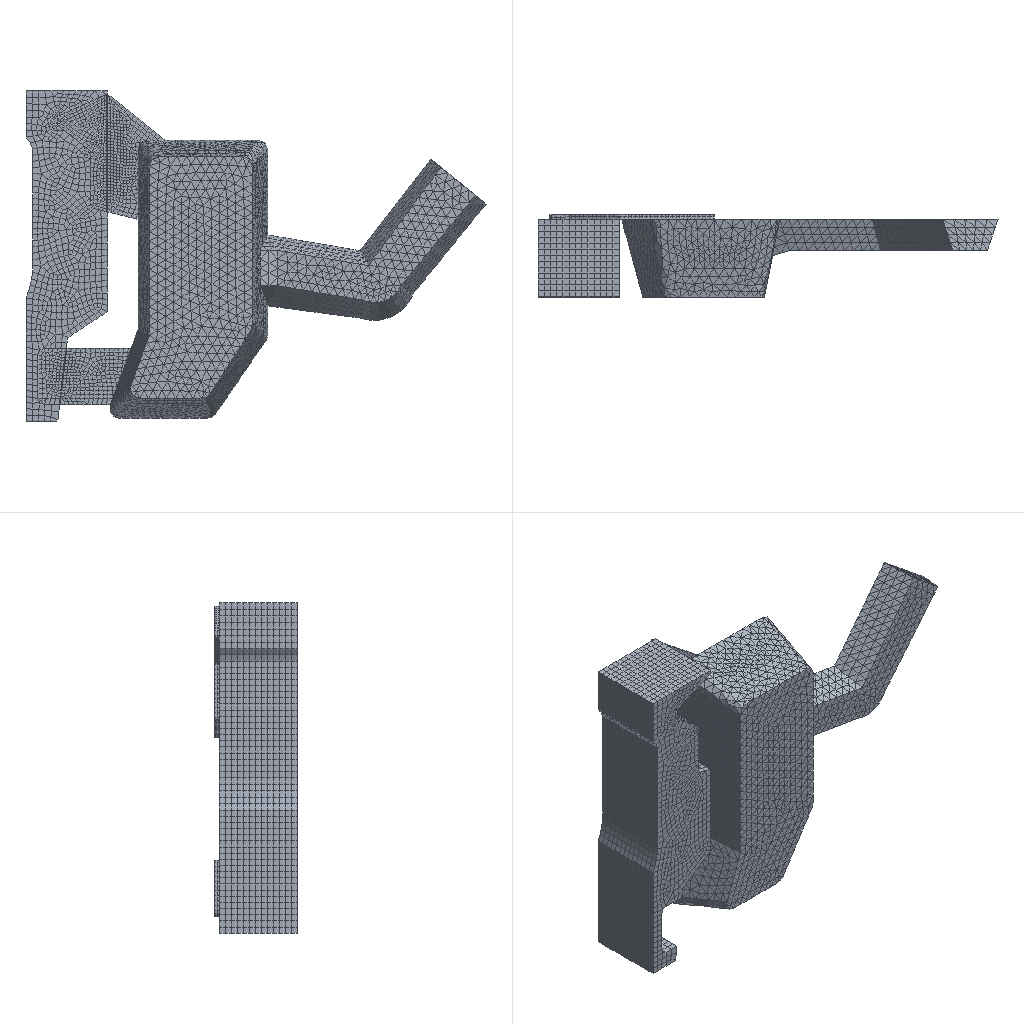Simulation study | abaqus
Set-up summary:
category,name,step,type,value,unit,region
solver,abaqus
solver,version,,,Abaqus/Explicit 2020
units,not stated in the deck,,not stated
analysis,deck,,transient,transient
load_step,Step-1,Step-1,transient,nlgeom=True
contact,interactions,,,general=1 pairs=0 ties=1
load_step,requested,,,1
mesh,nodes,,,20127
mesh,elements,,,40173
element_type,C3D4,,solid,29634
element_type,C3D8R,,solid,10483
element_type,COH3D8,,cohesive,56
load,load commands in deck,,count,1
bc,support commands in deck,,count,1
material,COH,,in results
material,MATERIAL-1,,in results
check,setup vs results,,match,"per instance, exact: element labels, types and connectivity; labels of the nodes the elements use; coordinates of those nodes at SINGLE_PRECISION in 2 of 3 instance(s)"
Abaqus input file, long lists of numbers shortened:
*Heading
** Job name: Job-1 Model name: Model-1
** Generated by: Abaqus/CAE 2020
*Preprint, echo=NO, model=NO, history=NO, contact=NO
**
** PARTS
**
*Part, name=work-1
*Node
      1,   552.966,         -10.,  -325.771
      2,   525.562,         -10.,  -321.176
** (6112 more lines like these left out)
*Element, type=C3D4
    1, 2263, 2264, 2265, 2266
    2, 2267, 2268, 2269, 2270
** (29632 more lines like these left out)
*Nset, nset=Set-4, generate
    1,  6114,     1
*Elset, elset=Set-4, generate
     1,  29634,      1
** Section: Section-1
*Solid Section, elset=Set-4, material=Material-1
,
*End Part
**
*Part, name=work-1-Copy
*Node
      1,   470.855,  0.8617,    -259.659
      2,   470.854,  0.8617,  -297.385
** (4547 more lines like these left out)
*Element, type=C3D8R
 1, 4472, 4473,  197,    7, 4475, 4474,  159,    4
 2, 4473, 4476,  198,  197, 4474, 4477,  158,  159
** (2694 more lines like these left out)
*Element, type=COH3D8
2697,   14,  358,  324,   13, 4437, 4436, 4435, 4434
2698,  358,  359,  323,  324, 4436, 4439, 4438, 4435
** (54 more lines like these left out)
*Nset, nset=Set-8, generate
    1,  4549,     1
*Elset, elset=Set-8, generate
    1,  2696,     1
*Elset, elset=CohesiveSeam-1-Elements, generate
 2697,  2752,     1
*Nset, nset=CohesiveSeam-1-TopNodes, generate
 4434,  4549,     1
*Nset, nset=CohesiveSeam-1-BottomNodes
   1,   2,   5,   8,  13,  14,  17,  18,  21,  86,  87,  88,  89,  90,  91,  92
  93,  94,  95,  96,  97,  98,  99, 100, 101, 102, 103, 104, 105, 106, 107, 108
** (6 more lines like these left out)
*Elset, elset=__PickedSurf18_S1, internal, generate
 2697,  2714,     1
*Elset, elset=__PickedSurf18_S2, internal, generate
 2715,  2752,     1
*Surface, type=ELEMENT, name=_PickedSurf18, internal
__PickedSurf18_S1, S1
__PickedSurf18_S2, S2
*Elset, elset=_CohesiveSeam-1-TopSurf_S2, internal, generate
 2697,  2752,     1
*Surface, type=ELEMENT, name=CohesiveSeam-1-TopSurf
_CohesiveSeam-1-TopSurf_S2, S2
*Elset, elset=_CohesiveSeam-1-BottomSurf_S1, internal, generate
 2697,  2752,     1
*Surface, type=ELEMENT, name=CohesiveSeam-1-BottomSurf
_CohesiveSeam-1-BottomSurf_S1, S1
** Section: Section-1
*Solid Section, elset=Set-8, material=Material-1
,
** Section: coh
*Cohesive Section, elset=CohesiveSeam-1-Elements, controls=EC-1, material=coh, response=TRACTION SEPARATION
,
*End Part
**
*Part, name=work-2
*Node
      1,   446.062,           0.,  -275.148
      2,   444.745,           0.,  -273.341
** (9462 more lines like these left out)
*Element, type=C3D8R
   1,  377,   89,    1,    3, 1053,  765,  677,  679
   2,   89,  371,    2,    1,  765, 1047,  678,  677
** (7785 more lines like these left out)
*Nset, nset=Set-1, generate
    1,  9464,     1
*Elset, elset=Set-1, generate
    1,  7787,     1
** Section: Section-1
*Solid Section, elset=Set-1, material=Material-1
,
*End Part
**
**
** ASSEMBLY
**
*Assembly, name=Assembly
**
*Instance, name=work-1-Copy-1, part=work-1-Copy
 -444.745,          25.,   258.5
*End Instance
**
*Instance, name=work-1-1, part=work-1
 -444.745,          25.,   258.5
*End Instance
**
*Instance, name=work-2-1, part=work-2
 -444.745,          25.,   258.5
*End Instance
**
*Node
      1,   77.674,          25.,  -57.725
*Nset, nset=Set-2, instance=work-2-1
    1,    2,    3,    4,    5,    6,    7,   67,   68,   69,   70,   71,   72,   73,   74,   75
   76,   77,   78,   79,   80,   81,   82,   83,   84,   85,  173,  174,  175,  215,  216,  217
** (46 more lines like these left out)
*Elset, elset=Set-2, instance=work-2-1
    1,    2,   19,   20,   21,   22,   23,   24,   25,   26,   27,   29,   32,   33,   37,   38
   40,   41,  150,  151,  158,  159,  160,  161,  162,  163,  164,  165,  166,  167,  168,  171
** (42 more lines like these left out)
*Nset, nset=Set-4
 1,
*Nset, nset=m_Set-3
 1,
*Elset, elset=_m_Surf-4_S2, internal, instance=work-1-Copy-1
 1231, 1232, 1233, 1234, 1235, 1236, 1237, 1238, 1239, 1240, 1241, 1242, 1243, 1244, 1245, 1246
 1247, 1248, 1249, 1250, 1251, 1252, 1253, 1254, 1255, 1256, 1257, 1258, 1259, 1260, 1261, 1262
** (53 more lines like these left out)
*Elset, elset=_m_Surf-4_S1, internal, instance=work-1-Copy-1, generate
  1,  76,   1
*Surface, type=ELEMENT, name=m_Surf-4
_m_Surf-4_S2, S2
_m_Surf-4_S1, S1
*Elset, elset=_m_Surf-6_S1, internal, instance=work-1-Copy-1
  95,  96,  97,  98,  99, 100, 101, 102, 103, 104, 105, 106, 107, 108, 109, 110
 111, 112, 113, 114, 115, 116, 117, 118, 119, 120, 121, 122, 123, 124, 125, 126
** (25 more lines like these left out)
*Elset, elset=_m_Surf-6_S4, internal, instance=work-1-Copy-1, generate
 77,  94,   1
*Elset, elset=_m_Surf-6_S6, internal, instance=work-1-Copy-1, generate
 735,  752,    1
*Surface, type=ELEMENT, name=m_Surf-6
_m_Surf-6_S1, S1
_m_Surf-6_S4, S4
_m_Surf-6_S6, S6
*Elset, elset=_m_Surf-8_S4, internal, instance=work-1-1
    19,  1446,  2491,  2536,  2958,  3117,  3520,  3581,  3606,  3731,  3771,  4246,  4450,  4540,  4760,  4968
  5013,  5272,  5591,  5704,  5708,  5733,  5749,  5763,  5808,  5919,  5922,  6552,  6559,  6565,  6602,  6980
** (3 more lines like these left out)
*Elset, elset=_m_Surf-8_S3, internal, instance=work-1-1
    25,   666,   805,  1207,  1254,  1332,  1847,  1898,  2482,  2515,  2555,  2576,  2597,  2602,  2619,  2643
  2645,  2646,  2668,  2669,  2672,  2673,  2674,  2686,  2690,  2696,  2714,  2719,  2735,  2737,  2746,  2773
** (69 more lines like these left out)
*Elset, elset=_m_Surf-8_S2, internal, instance=work-1-1
  2544,  2629,  3132,  3136,  3219,  3221,  3224,  3296,  3423,  3454,  3569,  3676,  3706,  3769,  3815,  3949
  4080,  4241,  4279,  4299,  4317,  4626,  4648,  4651,  4679,  4718,  4857,  4860,  4900,  5522,  5539,  5600
** (3 more lines like these left out)
*Elset, elset=_m_Surf-8_S1, internal, instance=work-1-1
  2560,  2975,  3284,  3580,  3612,  3644,  3842,  3975,  4142,  4179,  4235,  4634,  4923,  5500,  5558,  5603
  5609,  5635,  5642,  5748,  5925,  6589,  6663,  6713,  6714,  6717,  6725,  6731,  6757,  6784,  6815,  6841
** (2 more lines like these left out)
*Surface, type=ELEMENT, name=m_Surf-8
_m_Surf-8_S4, S4
_m_Surf-8_S3, S3
_m_Surf-8_S2, S2
_m_Surf-8_S1, S1
*Elset, elset=_s_Surf-4_S1, internal, instance=work-2-1, generate
   1,  599,    1
*Surface, type=ELEMENT, name=s_Surf-4
_s_Surf-4_S1, S1
*Elset, elset=_s_Surf-6_S1, internal, instance=work-2-1, generate
   1,  599,    1
*Surface, type=ELEMENT, name=s_Surf-6
_s_Surf-6_S1, S1
*Elset, elset=_s_Surf-8_S1, internal, instance=work-1-Copy-1
   1,   2,   3,   4,   5,   6,   7,   8,   9,  10,  11,  12,  13,  14,  15,  16
  17,  18,  19,  20,  21,  22,  23,  24,  25,  26,  27,  28,  29,  30,  31,  32
** (30 more lines like these left out)
*Elset, elset=_s_Surf-8_S4, internal, instance=work-1-Copy-1, generate
 77,  94,   1
*Elset, elset=_s_Surf-8_S6, internal, instance=work-1-Copy-1, generate
 735,  752,    1
*Elset, elset=_s_Surf-8_S2, internal, instance=work-1-Copy-1
 1231, 1232, 1233, 1234, 1235, 1236, 1237, 1238, 1239, 1240, 1241, 1242, 1243, 1244, 1245, 1246
 1247, 1248, 1249, 1250, 1251, 1252, 1253, 1254, 1255, 1256, 1257, 1258, 1259, 1260, 1261, 1262
** (53 more lines like these left out)
*Surface, type=ELEMENT, name=s_Surf-8
_s_Surf-8_S1, S1
_s_Surf-8_S4, S4
_s_Surf-8_S6, S6
_s_Surf-8_S2, S2
*Elset, elset=_s_Surf-10_S4, internal, instance=work-1-1
    19,  1446,  2491,  2536,  2958,  3117,  3520,  3581,  3606,  3731,  3771,  4246,  4450,  4540,  4760,  4968
  5013,  5272,  5591,  5704,  5708,  5733,  5749,  5763,  5808,  5919,  5922,  6552,  6559,  6565,  6602,  6980
** (3 more lines like these left out)
*Elset, elset=_s_Surf-10_S3, internal, instance=work-1-1
    25,   666,   805,  1207,  1254,  1332,  1847,  1898,  2482,  2515,  2555,  2576,  2597,  2602,  2619,  2643
  2645,  2646,  2668,  2669,  2672,  2673,  2674,  2686,  2690,  2696,  2714,  2719,  2735,  2737,  2746,  2773
** (69 more lines like these left out)
*Elset, elset=_s_Surf-10_S2, internal, instance=work-1-1
  2544,  2629,  3132,  3136,  3219,  3221,  3224,  3296,  3423,  3454,  3569,  3676,  3706,  3769,  3815,  3949
  4080,  4241,  4279,  4299,  4317,  4626,  4648,  4651,  4679,  4718,  4857,  4860,  4900,  5522,  5539,  5600
** (3 more lines like these left out)
*Elset, elset=_s_Surf-10_S1, internal, instance=work-1-1
  2560,  2975,  3284,  3580,  3612,  3644,  3842,  3975,  4142,  4179,  4235,  4634,  4923,  5500,  5558,  5603
  5609,  5635,  5642,  5748,  5925,  6589,  6663,  6713,  6714,  6717,  6725,  6731,  6757,  6784,  6815,  6841
** (2 more lines like these left out)
*Surface, type=ELEMENT, name=s_Surf-10
_s_Surf-10_S4, S4
_s_Surf-10_S3, S3
_s_Surf-10_S2, S2
_s_Surf-10_S1, S1
** Constraint: Constraint-1
*Tie, name=Constraint-1, adjust=yes
s_Surf-8, m_Surf-8
** Constraint: Constraint-2
*Coupling, constraint name=Constraint-2, ref node=m_Set-3, surface=s_Surf-10
*Kinematic
*End Assembly
**
** ELEMENT CONTROLS
**
*Section Controls, name=EC-1, ELEMENT DELETION=YES
1., 1., 1.
*Amplitude, name=Amp-1, definition=PERIODIC
1,             50.,              0.,              0.
             1.,              0.
**
** MATERIALS
**
*Material, name=Material-1
*Density
 2.7e-09,
*Elastic
69000., 0.3
*Material, name=coh
*Damage Initiation, criterion=MAXS
1.,1.,1.
*Damage Evolution, type=DISPLACEMENT
 1e-08,
*Density
 2.7e-09,
*Elastic, type=TRACTION
50000.,50000.,50000.
**
** INTERACTION PROPERTIES
**
*Surface Interaction, name=IntProp-1
*Friction
 0.15,
*Surface Behavior, pressure-overclosure=HARD
** ----------------------------------------------------------------
**
** STEP: Step-1
**
*Step, name=Step-1, nlgeom=YES
*Dynamic, Explicit
, 0.1
*Bulk Viscosity
0.06, 1.2
** Mass Scaling: Semi-Automatic
**               Whole Model
*Fixed Mass Scaling, factor=500.
**
** BOUNDARY CONDITIONS
**
** Name: BC-1 Type: 对称/反对称/完全固定
*Boundary
Set-2, ENCASTRE
**
** LOADS
**
** Name: Load-1   Type: Concentrated force
*Cload, amplitude=Amp-1
Set-4, 2, 300.
**
** INTERACTIONS
**
** Interaction: Int-3
*Contact, op=NEW
*Contact Inclusions, ALL EXTERIOR
*Contact Property Assignment
 ,  , IntProp-1
**
** OUTPUT REQUESTS
**
*Restart, write, number interval=1, time marks=NO
**
** FIELD OUTPUT: F-Output-1
**
*Output, field, number interval=50
*Node Output
A, CF, RF, RM, RT, U, V
*Element Output, directions=YES
E, EVF, LE, MISES, MISESMAX, PE, PEEQ, PEEQVAVG, PEVAVG, S, SDEG, SF, STATUS, SVAVG
*Contact Output
CDISP, CSTRESS
**
** HISTORY OUTPUT: H-Output-1
**
*Output, history, variable=PRESELECT
*End Step
Results summary:
result,step,Step-1,completed,increments=109789 time=0.1/0.1
result,analysis,,,transient
result,last_loadstep,,,1
result,analysis steps,,count,1
result,primary field,,,U
result,reaction total,,FX,-0.07608,model units
result,reaction total,,FY,0.7569,model units
result,reaction total,,FZ,-0.7432,model units